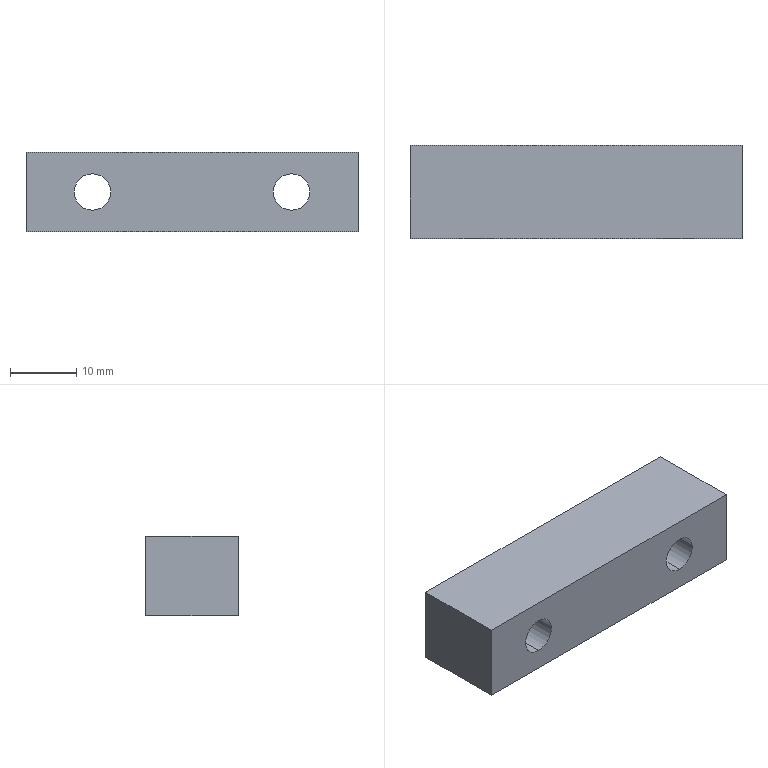Part | SolidWorks | features Extrusion 1, HoleWzd 1 | 1 solid | 16 faces | box 50 x 14 x 12 mm | volume 7110 mm3 | cylinder 8 | plane 8 | commonest cylinder face diameters 5.5 x4 10 x4
STEP:
#1=CARTESIAN_POINT('',(-15.,1.3,-5.));
#2=VERTEX_POINT('',#1);
#3=CARTESIAN_POINT('',(-15.,1.3,5.));
#4=VERTEX_POINT('',#3);
#5=CARTESIAN_POINT('',(-15.,1.3,0.));
#6=DIRECTION('',(0.,1.,0.));
#7=DIRECTION('',(0.,0.,1.));
#8=AXIS2_PLACEMENT_3D('',#5,#6,#7);
#9=CIRCLE('',#8,5.);
#10=EDGE_CURVE('',#2,#4,#9,.T.);
#11=ORIENTED_EDGE('',*,*,#10,.F.);
#12=CARTESIAN_POINT('',(-15.,7.,-5.));
#13=VERTEX_POINT('',#12);
#14=CARTESIAN_POINT('',(-15.,7.,-5.));
#15=DIRECTION('',(0.,1.,0.));
#16=VECTOR('',#15,1000.);
#17=LINE('',#14,#16);
#18=EDGE_CURVE('',#2,#13,#17,.T.);
#19=ORIENTED_EDGE('',*,*,#18,.T.);
#20=CARTESIAN_POINT('',(-15.,7.,5.));
#21=VERTEX_POINT('',#20);
#22=CARTESIAN_POINT('',(-15.,7.,0.));
#23=DIRECTION('',(0.,1.,0.));
#24=DIRECTION('',(0.,0.,1.));
#25=AXIS2_PLACEMENT_3D('',#22,#23,#24);
#26=CIRCLE('',#25,5.);
#27=EDGE_CURVE('',#13,#21,#26,.T.);
#28=ORIENTED_EDGE('',*,*,#27,.T.);
#29=CARTESIAN_POINT('',(-15.,7.,5.));
#30=DIRECTION('',(0.,1.,0.));
#31=VECTOR('',#30,1000.);
#32=LINE('',#29,#31);
#33=EDGE_CURVE('',#4,#21,#32,.T.);
#34=ORIENTED_EDGE('',*,*,#33,.F.);
#35=EDGE_LOOP('',(#11,#19,#28,#34));
#36=FACE_OUTER_BOUND('',#35,.T.);
#37=CARTESIAN_POINT('',(-15.,7.,0.));
#38=DIRECTION('',(0.,1.,0.));
#39=DIRECTION('',(0.,0.,1.));
#40=AXIS2_PLACEMENT_3D('',#37,#38,#39);
#41=CYLINDRICAL_SURFACE('',#40,5.);
#42=ADVANCED_FACE('',(#36),#41,.F.);
#43=CARTESIAN_POINT('',(-15.,-7.,-2.75));
#44=VERTEX_POINT('',#43);
#45=CARTESIAN_POINT('',(-15.,-7.,2.75));
#46=VERTEX_POINT('',#45);
#47=CARTESIAN_POINT('',(-15.,-7.,0.));
#48=DIRECTION('',(0.,1.,0.));
#49=DIRECTION('',(0.,0.,1.));
#50=AXIS2_PLACEMENT_3D('',#47,#48,#49);
#51=CIRCLE('',#50,2.75);
#52=EDGE_CURVE('',#44,#46,#51,.T.);
#53=ORIENTED_EDGE('',*,*,#52,.F.);
#54=CARTESIAN_POINT('',(-15.,1.3,-2.75));
#55=VERTEX_POINT('',#54);
#56=CARTESIAN_POINT('',(-15.,7.,-2.75));
#57=DIRECTION('',(0.,1.,0.));
#58=VECTOR('',#57,1000.);
#59=LINE('',#56,#58);
#60=EDGE_CURVE('',#44,#55,#59,.T.);
#61=ORIENTED_EDGE('',*,*,#60,.T.);
#62=CARTESIAN_POINT('',(-15.,1.3,2.75));
#63=VERTEX_POINT('',#62);
#64=CARTESIAN_POINT('',(-15.,1.3,0.));
#65=DIRECTION('',(0.,1.,0.));
#66=DIRECTION('',(0.,0.,1.));
#67=AXIS2_PLACEMENT_3D('',#64,#65,#66);
#68=CIRCLE('',#67,2.75);
#69=EDGE_CURVE('',#55,#63,#68,.T.);
#70=ORIENTED_EDGE('',*,*,#69,.T.);
#71=CARTESIAN_POINT('',(-15.,7.,2.75));
#72=DIRECTION('',(0.,1.,0.));
#73=VECTOR('',#72,1000.);
#74=LINE('',#71,#73);
#75=EDGE_CURVE('',#46,#63,#74,.T.);
#76=ORIENTED_EDGE('',*,*,#75,.F.);
#77=EDGE_LOOP('',(#53,#61,#70,#76));
#78=FACE_OUTER_BOUND('',#77,.T.);
#79=CARTESIAN_POINT('',(-15.,7.,0.));
#80=DIRECTION('',(0.,1.,0.));
#81=DIRECTION('',(0.,0.,1.));
#82=AXIS2_PLACEMENT_3D('',#79,#80,#81);
#83=CYLINDRICAL_SURFACE('',#82,2.75);
#84=ADVANCED_FACE('',(#78),#83,.F.);
#85=CARTESIAN_POINT('',(15.,1.3,-5.));
#86=VERTEX_POINT('',#85);
#87=CARTESIAN_POINT('',(15.,1.3,5.));
#88=VERTEX_POINT('',#87);
#89=CARTESIAN_POINT('',(15.,1.3,0.));
#90=DIRECTION('',(0.,1.,0.));
#91=DIRECTION('',(0.,0.,1.));
#92=AXIS2_PLACEMENT_3D('',#89,#90,#91);
#93=CIRCLE('',#92,5.);
#94=EDGE_CURVE('',#86,#88,#93,.T.);
#95=ORIENTED_EDGE('',*,*,#94,.F.);
#96=CARTESIAN_POINT('',(15.,7.,-5.));
#97=VERTEX_POINT('',#96);
#98=CARTESIAN_POINT('',(15.,7.,-5.));
#99=DIRECTION('',(0.,1.,0.));
#100=VECTOR('',#99,1000.);
#101=LINE('',#98,#100);
#102=EDGE_CURVE('',#86,#97,#101,.T.);
#103=ORIENTED_EDGE('',*,*,#102,.T.);
#104=CARTESIAN_POINT('',(15.,7.,5.));
#105=VERTEX_POINT('',#104);
#106=CARTESIAN_POINT('',(15.,7.,0.));
#107=DIRECTION('',(0.,1.,0.));
#108=DIRECTION('',(0.,0.,1.));
#109=AXIS2_PLACEMENT_3D('',#106,#107,#108);
#110=CIRCLE('',#109,5.);
#111=EDGE_CURVE('',#97,#105,#110,.T.);
#112=ORIENTED_EDGE('',*,*,#111,.T.);
#113=CARTESIAN_POINT('',(15.,7.,5.));
#114=DIRECTION('',(0.,1.,0.));
#115=VECTOR('',#114,1000.);
#116=LINE('',#113,#115);
#117=EDGE_CURVE('',#88,#105,#116,.T.);
#118=ORIENTED_EDGE('',*,*,#117,.F.);
#119=EDGE_LOOP('',(#95,#103,#112,#118));
#120=FACE_OUTER_BOUND('',#119,.T.);
#121=CARTESIAN_POINT('',(15.,7.,0.));
#122=DIRECTION('',(0.,1.,0.));
#123=DIRECTION('',(0.,0.,1.));
#124=AXIS2_PLACEMENT_3D('',#121,#122,#123);
#125=CYLINDRICAL_SURFACE('',#124,5.);
#126=ADVANCED_FACE('',(#120),#125,.F.);
#127=CARTESIAN_POINT('',(15.,-7.,-2.75));
#128=VERTEX_POINT('',#127);
#129=CARTESIAN_POINT('',(15.,-7.,2.75));
#130=VERTEX_POINT('',#129);
#131=CARTESIAN_POINT('',(15.,-7.,0.));
#132=DIRECTION('',(0.,1.,0.));
#133=DIRECTION('',(0.,0.,1.));
#134=AXIS2_PLACEMENT_3D('',#131,#132,#133);
#135=CIRCLE('',#134,2.75);
#136=EDGE_CURVE('',#128,#130,#135,.T.);
#137=ORIENTED_EDGE('',*,*,#136,.F.);
#138=CARTESIAN_POINT('',(15.,1.3,-2.75));
#139=VERTEX_POINT('',#138);
#140=CARTESIAN_POINT('',(15.,7.,-2.75));
#141=DIRECTION('',(0.,1.,0.));
#142=VECTOR('',#141,1000.);
#143=LINE('',#140,#142);
#144=EDGE_CURVE('',#128,#139,#143,.T.);
#145=ORIENTED_EDGE('',*,*,#144,.T.);
#146=CARTESIAN_POINT('',(15.,1.3,2.75));
#147=VERTEX_POINT('',#146);
#148=CARTESIAN_POINT('',(15.,1.3,0.));
#149=DIRECTION('',(0.,1.,0.));
#150=DIRECTION('',(0.,0.,1.));
#151=AXIS2_PLACEMENT_3D('',#148,#149,#150);
#152=CIRCLE('',#151,2.75);
#153=EDGE_CURVE('',#139,#147,#152,.T.);
#154=ORIENTED_EDGE('',*,*,#153,.T.);
#155=CARTESIAN_POINT('',(15.,7.,2.75));
#156=DIRECTION('',(0.,1.,0.));
#157=VECTOR('',#156,1000.);
#158=LINE('',#155,#157);
#159=EDGE_CURVE('',#130,#147,#158,.T.);
#160=ORIENTED_EDGE('',*,*,#159,.F.);
#161=EDGE_LOOP('',(#137,#145,#154,#160));
#162=FACE_OUTER_BOUND('',#161,.T.);
#163=CARTESIAN_POINT('',(15.,7.,0.));
#164=DIRECTION('',(0.,1.,0.));
#165=DIRECTION('',(0.,0.,1.));
#166=AXIS2_PLACEMENT_3D('',#163,#164,#165);
#167=CYLINDRICAL_SURFACE('',#166,2.75);
#168=ADVANCED_FACE('',(#162),#167,.F.);
#169=CARTESIAN_POINT('',(25.,-7.,6.));
#170=VERTEX_POINT('',#169);
#171=CARTESIAN_POINT('',(25.,-7.,-6.));
#172=VERTEX_POINT('',#171);
#173=CARTESIAN_POINT('',(25.,-7.,6.));
#174=DIRECTION('',(0.,0.,-1.));
#175=VECTOR('',#174,1000.);
#176=LINE('',#173,#175);
#177=EDGE_CURVE('',#170,#172,#176,.T.);
#178=ORIENTED_EDGE('',*,*,#177,.T.);
#179=CARTESIAN_POINT('',(25.,7.,-6.));
#180=VERTEX_POINT('',#179);
#181=CARTESIAN_POINT('',(25.,7.,-6.));
#182=DIRECTION('',(0.,-1.,0.));
#183=VECTOR('',#182,1000.);
#184=LINE('',#181,#183);
#185=EDGE_CURVE('',#180,#172,#184,.T.);
#186=ORIENTED_EDGE('',*,*,#185,.F.);
#187=CARTESIAN_POINT('',(25.,7.,6.));
#188=VERTEX_POINT('',#187);
#189=CARTESIAN_POINT('',(25.,7.,6.));
#190=DIRECTION('',(0.,0.,-1.));
#191=VECTOR('',#190,1000.);
#192=LINE('',#189,#191);
#193=EDGE_CURVE('',#188,#180,#192,.T.);
#194=ORIENTED_EDGE('',*,*,#193,.F.);
#195=CARTESIAN_POINT('',(25.,7.,6.));
#196=DIRECTION('',(0.,-1.,0.));
#197=VECTOR('',#196,1000.);
#198=LINE('',#195,#197);
#199=EDGE_CURVE('',#188,#170,#198,.T.);
#200=ORIENTED_EDGE('',*,*,#199,.T.);
#201=EDGE_LOOP('',(#178,#186,#194,#200));
#202=FACE_OUTER_BOUND('',#201,.T.);
#203=CARTESIAN_POINT('',(25.,7.,6.));
#204=DIRECTION('',(-1.,0.,0.));
#205=DIRECTION('',(0.,0.,1.));
#206=AXIS2_PLACEMENT_3D('',#203,#204,#205);
#207=PLANE('',#206);
#208=ADVANCED_FACE('',(#202),#207,.F.);
#209=CARTESIAN_POINT('',(-25.,-7.,-6.));
#210=VERTEX_POINT('',#209);
#211=CARTESIAN_POINT('',(-25.,-7.,-6.));
#212=DIRECTION('',(-1.,0.,0.));
#213=VECTOR('',#212,1000.);
#214=LINE('',#211,#213);
#215=EDGE_CURVE('',#172,#210,#214,.T.);
#216=ORIENTED_EDGE('',*,*,#215,.T.);
#217=CARTESIAN_POINT('',(-25.,7.,-6.));
#218=VERTEX_POINT('',#217);
#219=CARTESIAN_POINT('',(-25.,7.,-6.));
#220=DIRECTION('',(0.,-1.,0.));
#221=VECTOR('',#220,1000.);
#222=LINE('',#219,#221);
#223=EDGE_CURVE('',#218,#210,#222,.T.);
#224=ORIENTED_EDGE('',*,*,#223,.F.);
#225=CARTESIAN_POINT('',(-25.,7.,-6.));
#226=DIRECTION('',(-1.,0.,0.));
#227=VECTOR('',#226,1000.);
#228=LINE('',#225,#227);
#229=EDGE_CURVE('',#180,#218,#228,.T.);
#230=ORIENTED_EDGE('',*,*,#229,.F.);
#231=ORIENTED_EDGE('',*,*,#185,.T.);
#232=EDGE_LOOP('',(#216,#224,#230,#231));
#233=FACE_OUTER_BOUND('',#232,.T.);
#234=CARTESIAN_POINT('',(-25.,7.,-6.));
#235=DIRECTION('',(0.,0.,1.));
#236=DIRECTION('',(1.,0.,0.));
#237=AXIS2_PLACEMENT_3D('',#234,#235,#236);
#238=PLANE('',#237);
#239=ADVANCED_FACE('',(#233),#238,.F.);
#240=CARTESIAN_POINT('',(-25.,-7.,6.));
#241=VERTEX_POINT('',#240);
#242=CARTESIAN_POINT('',(-25.,-7.,6.));
#243=DIRECTION('',(0.,0.,1.));
#244=VECTOR('',#243,1000.);
#245=LINE('',#242,#244);
#246=EDGE_CURVE('',#210,#241,#245,.T.);
#247=ORIENTED_EDGE('',*,*,#246,.T.);
#248=CARTESIAN_POINT('',(-25.,7.,6.));
#249=VERTEX_POINT('',#248);
#250=CARTESIAN_POINT('',(-25.,7.,6.));
#251=DIRECTION('',(0.,-1.,0.));
#252=VECTOR('',#251,1000.);
#253=LINE('',#250,#252);
#254=EDGE_CURVE('',#249,#241,#253,.T.);
#255=ORIENTED_EDGE('',*,*,#254,.F.);
#256=CARTESIAN_POINT('',(-25.,7.,6.));
#257=DIRECTION('',(0.,0.,1.));
#258=VECTOR('',#257,1000.);
#259=LINE('',#256,#258);
#260=EDGE_CURVE('',#218,#249,#259,.T.);
#261=ORIENTED_EDGE('',*,*,#260,.F.);
#262=ORIENTED_EDGE('',*,*,#223,.T.);
#263=EDGE_LOOP('',(#247,#255,#261,#262));
#264=FACE_OUTER_BOUND('',#263,.T.);
#265=CARTESIAN_POINT('',(-25.,7.,6.));
#266=DIRECTION('',(1.,0.,0.));
#267=DIRECTION('',(0.,0.,-1.));
#268=AXIS2_PLACEMENT_3D('',#265,#266,#267);
#269=PLANE('',#268);
#270=ADVANCED_FACE('',(#264),#269,.F.);
#271=CARTESIAN_POINT('',(-25.,-7.,6.));
#272=DIRECTION('',(1.,0.,0.));
#273=VECTOR('',#272,1000.);
#274=LINE('',#271,#273);
#275=EDGE_CURVE('',#241,#170,#274,.T.);
#276=ORIENTED_EDGE('',*,*,#275,.T.);
#277=ORIENTED_EDGE('',*,*,#199,.F.);
#278=CARTESIAN_POINT('',(-25.,7.,6.));
#279=DIRECTION('',(1.,0.,0.));
#280=VECTOR('',#279,1000.);
#281=LINE('',#278,#280);
#282=EDGE_CURVE('',#249,#188,#281,.T.);
#283=ORIENTED_EDGE('',*,*,#282,.F.);
#284=ORIENTED_EDGE('',*,*,#254,.T.);
#285=EDGE_LOOP('',(#276,#277,#283,#284));
#286=FACE_OUTER_BOUND('',#285,.T.);
#287=CARTESIAN_POINT('',(-25.,7.,6.));
#288=DIRECTION('',(0.,0.,-1.));
#289=DIRECTION('',(-1.,0.,0.));
#290=AXIS2_PLACEMENT_3D('',#287,#288,#289);
#291=PLANE('',#290);
#292=ADVANCED_FACE('',(#286),#291,.F.);
#293=CARTESIAN_POINT('',(-15.,7.,0.));
#294=DIRECTION('',(0.,1.,0.));
#295=DIRECTION('',(0.,0.,1.));
#296=AXIS2_PLACEMENT_3D('',#293,#294,#295);
#297=CIRCLE('',#296,5.);
#298=EDGE_CURVE('',#21,#13,#297,.T.);
#299=ORIENTED_EDGE('',*,*,#298,.F.);
#300=ORIENTED_EDGE('',*,*,#27,.F.);
#301=EDGE_LOOP('',(#299,#300));
#302=FACE_BOUND('',#301,.T.);
#303=CARTESIAN_POINT('',(15.,7.,0.));
#304=DIRECTION('',(0.,1.,0.));
#305=DIRECTION('',(0.,0.,1.));
#306=AXIS2_PLACEMENT_3D('',#303,#304,#305);
#307=CIRCLE('',#306,5.);
#308=EDGE_CURVE('',#105,#97,#307,.T.);
#309=ORIENTED_EDGE('',*,*,#308,.F.);
#310=ORIENTED_EDGE('',*,*,#111,.F.);
#311=EDGE_LOOP('',(#309,#310));
#312=FACE_BOUND('',#311,.T.);
#313=ORIENTED_EDGE('',*,*,#193,.T.);
#314=ORIENTED_EDGE('',*,*,#229,.T.);
#315=ORIENTED_EDGE('',*,*,#260,.T.);
#316=ORIENTED_EDGE('',*,*,#282,.T.);
#317=EDGE_LOOP('',(#313,#314,#315,#316));
#318=FACE_OUTER_BOUND('',#317,.T.);
#319=CARTESIAN_POINT('',(0.,7.,0.));
#320=DIRECTION('',(0.,-1.,0.));
#321=DIRECTION('',(0.,0.,-1.));
#322=AXIS2_PLACEMENT_3D('',#319,#320,#321);
#323=PLANE('',#322);
#324=ADVANCED_FACE('',(#302,#312,#318),#323,.F.);
#325=CARTESIAN_POINT('',(-15.,-7.,0.));
#326=DIRECTION('',(0.,1.,0.));
#327=DIRECTION('',(0.,0.,1.));
#328=AXIS2_PLACEMENT_3D('',#325,#326,#327);
#329=CIRCLE('',#328,2.75);
#330=EDGE_CURVE('',#46,#44,#329,.T.);
#331=ORIENTED_EDGE('',*,*,#330,.T.);
#332=ORIENTED_EDGE('',*,*,#52,.T.);
#333=EDGE_LOOP('',(#331,#332));
#334=FACE_BOUND('',#333,.T.);
#335=CARTESIAN_POINT('',(15.,-7.,0.));
#336=DIRECTION('',(0.,1.,0.));
#337=DIRECTION('',(0.,0.,1.));
#338=AXIS2_PLACEMENT_3D('',#335,#336,#337);
#339=CIRCLE('',#338,2.75);
#340=EDGE_CURVE('',#130,#128,#339,.T.);
#341=ORIENTED_EDGE('',*,*,#340,.T.);
#342=ORIENTED_EDGE('',*,*,#136,.T.);
#343=EDGE_LOOP('',(#341,#342));
#344=FACE_BOUND('',#343,.T.);
#345=ORIENTED_EDGE('',*,*,#177,.F.);
#346=ORIENTED_EDGE('',*,*,#275,.F.);
#347=ORIENTED_EDGE('',*,*,#246,.F.);
#348=ORIENTED_EDGE('',*,*,#215,.F.);
#349=EDGE_LOOP('',(#345,#346,#347,#348));
#350=FACE_OUTER_BOUND('',#349,.T.);
#351=CARTESIAN_POINT('',(0.,-7.,0.));
#352=DIRECTION('',(0.,-1.,0.));
#353=DIRECTION('',(0.,0.,-1.));
#354=AXIS2_PLACEMENT_3D('',#351,#352,#353);
#355=PLANE('',#354);
#356=ADVANCED_FACE('',(#334,#344,#350),#355,.T.);
#357=ORIENTED_EDGE('',*,*,#144,.F.);
#358=ORIENTED_EDGE('',*,*,#340,.F.);
#359=ORIENTED_EDGE('',*,*,#159,.T.);
#360=CARTESIAN_POINT('',(15.,1.3,0.));
#361=DIRECTION('',(0.,1.,0.));
#362=DIRECTION('',(0.,0.,1.));
#363=AXIS2_PLACEMENT_3D('',#360,#361,#362);
#364=CIRCLE('',#363,2.75);
#365=EDGE_CURVE('',#147,#139,#364,.T.);
#366=ORIENTED_EDGE('',*,*,#365,.T.);
#367=EDGE_LOOP('',(#357,#358,#359,#366));
#368=FACE_OUTER_BOUND('',#367,.T.);
#369=CARTESIAN_POINT('',(15.,7.,0.));
#370=DIRECTION('',(0.,1.,0.));
#371=DIRECTION('',(0.,0.,1.));
#372=AXIS2_PLACEMENT_3D('',#369,#370,#371);
#373=CYLINDRICAL_SURFACE('',#372,2.75);
#374=ADVANCED_FACE('',(#368),#373,.F.);
#375=ORIENTED_EDGE('',*,*,#365,.F.);
#376=ORIENTED_EDGE('',*,*,#153,.F.);
#377=EDGE_LOOP('',(#375,#376));
#378=FACE_BOUND('',#377,.T.);
#379=CARTESIAN_POINT('',(15.,1.3,0.));
#380=DIRECTION('',(0.,1.,0.));
#381=DIRECTION('',(0.,0.,1.));
#382=AXIS2_PLACEMENT_3D('',#379,#380,#381);
#383=CIRCLE('',#382,5.);
#384=EDGE_CURVE('',#88,#86,#383,.T.);
#385=ORIENTED_EDGE('',*,*,#384,.T.);
#386=ORIENTED_EDGE('',*,*,#94,.T.);
#387=EDGE_LOOP('',(#385,#386));
#388=FACE_OUTER_BOUND('',#387,.T.);
#389=CARTESIAN_POINT('',(17.75,1.3,0.));
#390=DIRECTION('',(0.,-1.,0.));
#391=DIRECTION('',(0.,0.,-1.));
#392=AXIS2_PLACEMENT_3D('',#389,#390,#391);
#393=PLANE('',#392);
#394=ADVANCED_FACE('',(#378,#388),#393,.F.);
#395=ORIENTED_EDGE('',*,*,#102,.F.);
#396=ORIENTED_EDGE('',*,*,#384,.F.);
#397=ORIENTED_EDGE('',*,*,#117,.T.);
#398=ORIENTED_EDGE('',*,*,#308,.T.);
#399=EDGE_LOOP('',(#395,#396,#397,#398));
#400=FACE_OUTER_BOUND('',#399,.T.);
#401=CARTESIAN_POINT('',(15.,7.,0.));
#402=DIRECTION('',(0.,1.,0.));
#403=DIRECTION('',(0.,0.,1.));
#404=AXIS2_PLACEMENT_3D('',#401,#402,#403);
#405=CYLINDRICAL_SURFACE('',#404,5.);
#406=ADVANCED_FACE('',(#400),#405,.F.);
#407=ORIENTED_EDGE('',*,*,#60,.F.);
#408=ORIENTED_EDGE('',*,*,#330,.F.);
#409=ORIENTED_EDGE('',*,*,#75,.T.);
#410=CARTESIAN_POINT('',(-15.,1.3,0.));
#411=DIRECTION('',(0.,1.,0.));
#412=DIRECTION('',(0.,0.,1.));
#413=AXIS2_PLACEMENT_3D('',#410,#411,#412);
#414=CIRCLE('',#413,2.75);
#415=EDGE_CURVE('',#63,#55,#414,.T.);
#416=ORIENTED_EDGE('',*,*,#415,.T.);
#417=EDGE_LOOP('',(#407,#408,#409,#416));
#418=FACE_OUTER_BOUND('',#417,.T.);
#419=CARTESIAN_POINT('',(-15.,7.,0.));
#420=DIRECTION('',(0.,1.,0.));
#421=DIRECTION('',(0.,0.,1.));
#422=AXIS2_PLACEMENT_3D('',#419,#420,#421);
#423=CYLINDRICAL_SURFACE('',#422,2.75);
#424=ADVANCED_FACE('',(#418),#423,.F.);
#425=ORIENTED_EDGE('',*,*,#415,.F.);
#426=ORIENTED_EDGE('',*,*,#69,.F.);
#427=EDGE_LOOP('',(#425,#426));
#428=FACE_BOUND('',#427,.T.);
#429=CARTESIAN_POINT('',(-15.,1.3,0.));
#430=DIRECTION('',(0.,1.,0.));
#431=DIRECTION('',(0.,0.,1.));
#432=AXIS2_PLACEMENT_3D('',#429,#430,#431);
#433=CIRCLE('',#432,5.);
#434=EDGE_CURVE('',#4,#2,#433,.T.);
#435=ORIENTED_EDGE('',*,*,#434,.T.);
#436=ORIENTED_EDGE('',*,*,#10,.T.);
#437=EDGE_LOOP('',(#435,#436));
#438=FACE_OUTER_BOUND('',#437,.T.);
#439=CARTESIAN_POINT('',(-12.25,1.3,0.));
#440=DIRECTION('',(0.,-1.,0.));
#441=DIRECTION('',(0.,0.,-1.));
#442=AXIS2_PLACEMENT_3D('',#439,#440,#441);
#443=PLANE('',#442);
#444=ADVANCED_FACE('',(#428,#438),#443,.F.);
#445=ORIENTED_EDGE('',*,*,#18,.F.);
#446=ORIENTED_EDGE('',*,*,#434,.F.);
#447=ORIENTED_EDGE('',*,*,#33,.T.);
#448=ORIENTED_EDGE('',*,*,#298,.T.);
#449=EDGE_LOOP('',(#445,#446,#447,#448));
#450=FACE_OUTER_BOUND('',#449,.T.);
#451=CARTESIAN_POINT('',(-15.,7.,0.));
#452=DIRECTION('',(0.,1.,0.));
#453=DIRECTION('',(0.,0.,1.));
#454=AXIS2_PLACEMENT_3D('',#451,#452,#453);
#455=CYLINDRICAL_SURFACE('',#454,5.);
#456=ADVANCED_FACE('',(#450),#455,.F.);
#457=CLOSED_SHELL('',(#42,#84,#126,#168,#208,#239,#270,#292,#324,#356,#374,#394,#406,#424,#444,#456));
#458=MANIFOLD_SOLID_BREP('',#457);
#459=CARTESIAN_POINT('',(0.,0.,0.));
#460=DIRECTION('',(0.,0.,1.));
#461=DIRECTION('',(1.,0.,0.));
#462=AXIS2_PLACEMENT_3D('',#459,#460,#461);
#463=(LENGTH_UNIT()NAMED_UNIT(*)SI_UNIT(.MILLI.,.METRE.));
#464=UNCERTAINTY_MEASURE_WITH_UNIT(LENGTH_MEASURE(0.00001),#463,'','');
#465=(NAMED_UNIT(*)PLANE_ANGLE_UNIT()SI_UNIT($,.RADIAN.));
#466=(NAMED_UNIT(*)SI_UNIT($,.STERADIAN.)SOLID_ANGLE_UNIT());
#467=(GEOMETRIC_REPRESENTATION_CONTEXT(3)GLOBAL_UNCERTAINTY_ASSIGNED_CONTEXT((#464))GLOBAL_UNIT_ASSIGNED_CONTEXT((#463,#465,#466))REPRESENTATION_CONTEXT('',''));
#468=ADVANCED_BREP_SHAPE_REPRESENTATION('',(#458,#462),#467);